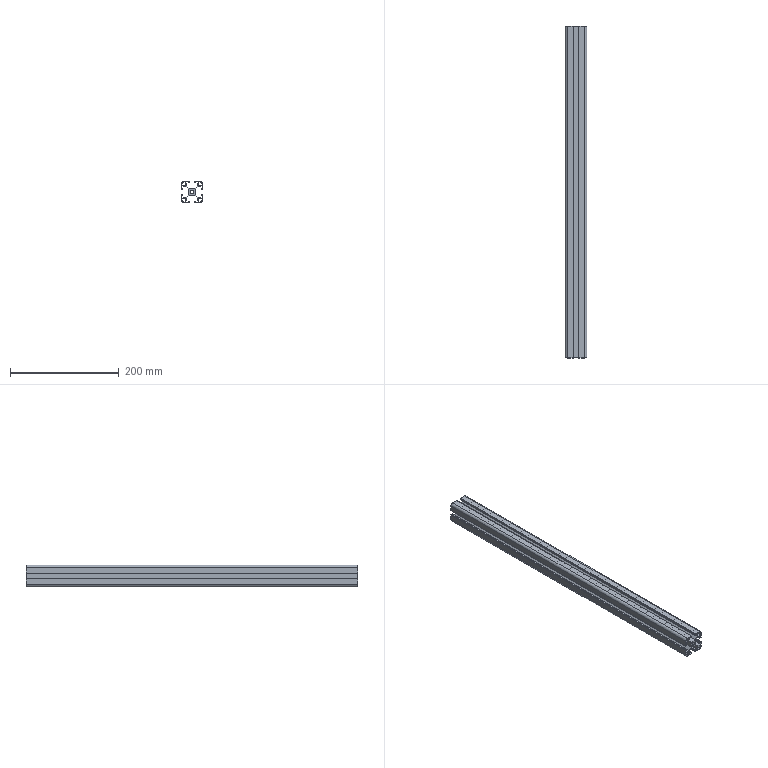Part | SolidWorks | features BaseBody 1 | 1 solid | 104 faces | box 40 x 610 x 40 mm | volume 289668 mm3 | plane 94 | cylinder 10 | commonest cylinder face diameters 5 x4 9 x4 6.8 x2